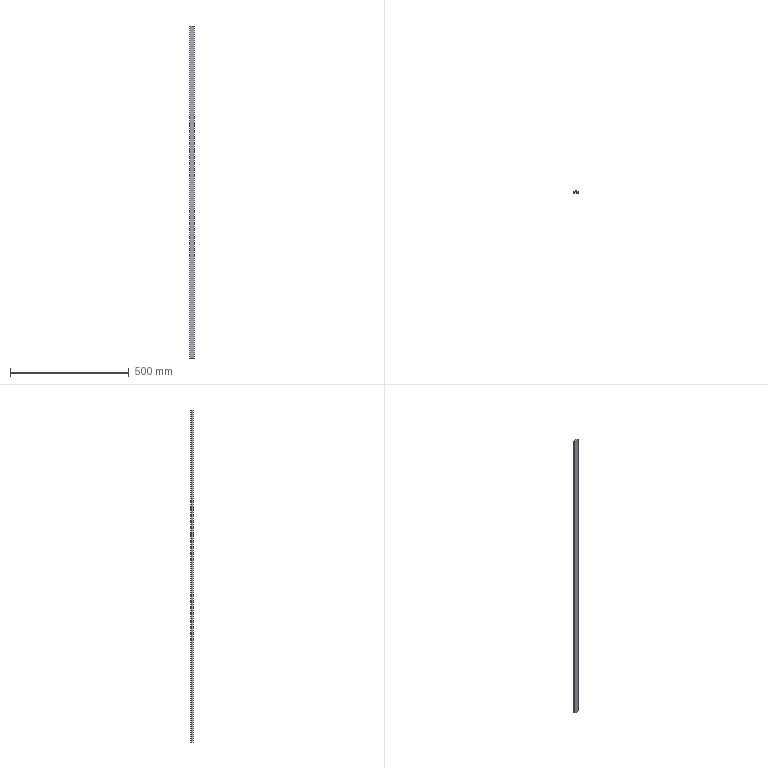Part | STEP file | GDT40-2000 | 1 solid | 10 faces | box 20 x 10 x 1400 mm | volume 237664 mm3 | plane 10
STEP:
#1=CARTESIAN_POINT('',(3.7,10.,400.));
#2=VERTEX_POINT('',#1);
#3=CARTESIAN_POINT('',(3.7,10.,-1000.));
#4=VERTEX_POINT('',#3);
#5=CARTESIAN_POINT('',(3.7,10.,1000.));
#6=DIRECTION('',(0.,0.,-1.));
#7=VECTOR('',#6,1000.);
#8=LINE('',#5,#7);
#9=EDGE_CURVE('',#2,#4,#8,.T.);
#10=ORIENTED_EDGE('',*,*,#9,.F.);
#11=CARTESIAN_POINT('',(3.7,7.6,400.));
#12=VERTEX_POINT('',#11);
#13=CARTESIAN_POINT('',(3.7,7.6,400.));
#14=DIRECTION('',(0.,1.,0.));
#15=VECTOR('',#14,1000.);
#16=LINE('',#13,#15);
#17=EDGE_CURVE('',#12,#2,#16,.T.);
#18=ORIENTED_EDGE('',*,*,#17,.F.);
#19=CARTESIAN_POINT('',(3.7,7.6,-1000.));
#20=VERTEX_POINT('',#19);
#21=CARTESIAN_POINT('',(3.7,7.6,1000.));
#22=DIRECTION('',(0.,0.,1.));
#23=VECTOR('',#22,1000.);
#24=LINE('',#21,#23);
#25=EDGE_CURVE('',#20,#12,#24,.T.);
#26=ORIENTED_EDGE('',*,*,#25,.F.);
#27=CARTESIAN_POINT('',(3.7,0.,-1000.));
#28=DIRECTION('',(0.,1.,0.));
#29=VECTOR('',#28,1000.);
#30=LINE('',#27,#29);
#31=EDGE_CURVE('',#20,#4,#30,.T.);
#32=ORIENTED_EDGE('',*,*,#31,.T.);
#33=EDGE_LOOP('',(#10,#18,#26,#32));
#34=FACE_OUTER_BOUND('',#33,.T.);
#35=CARTESIAN_POINT('',(3.7,7.6,1000.));
#36=DIRECTION('',(1.,0.,0.));
#37=DIRECTION('',(0.,0.,-1.));
#38=AXIS2_PLACEMENT_3D('',#35,#36,#37);
#39=PLANE('',#38);
#40=ADVANCED_FACE('',(#34),#39,.T.);
#41=CARTESIAN_POINT('',(-3.7,10.,400.));
#42=VERTEX_POINT('',#41);
#43=CARTESIAN_POINT('',(-3.7,10.,-1000.));
#44=VERTEX_POINT('',#43);
#45=CARTESIAN_POINT('',(-3.7,10.,1000.));
#46=DIRECTION('',(0.,0.,-1.));
#47=VECTOR('',#46,1000.);
#48=LINE('',#45,#47);
#49=EDGE_CURVE('',#42,#44,#48,.T.);
#50=ORIENTED_EDGE('',*,*,#49,.F.);
#51=CARTESIAN_POINT('',(3.7,10.,400.));
#52=DIRECTION('',(-1.,0.,0.));
#53=VECTOR('',#52,1000.);
#54=LINE('',#51,#53);
#55=EDGE_CURVE('',#2,#42,#54,.T.);
#56=ORIENTED_EDGE('',*,*,#55,.F.);
#57=ORIENTED_EDGE('',*,*,#9,.T.);
#58=CARTESIAN_POINT('',(0.,10.,-1000.));
#59=DIRECTION('',(-1.,0.,0.));
#60=VECTOR('',#59,1000.);
#61=LINE('',#58,#60);
#62=EDGE_CURVE('',#4,#44,#61,.T.);
#63=ORIENTED_EDGE('',*,*,#62,.T.);
#64=EDGE_LOOP('',(#50,#56,#57,#63));
#65=FACE_OUTER_BOUND('',#64,.T.);
#66=CARTESIAN_POINT('',(3.7,10.,1000.));
#67=DIRECTION('',(0.,1.,0.));
#68=DIRECTION('',(0.,0.,1.));
#69=AXIS2_PLACEMENT_3D('',#66,#67,#68);
#70=PLANE('',#69);
#71=ADVANCED_FACE('',(#65),#70,.T.);
#72=CARTESIAN_POINT('',(-3.7,7.6,400.));
#73=VERTEX_POINT('',#72);
#74=CARTESIAN_POINT('',(-3.7,7.6,-1000.));
#75=VERTEX_POINT('',#74);
#76=CARTESIAN_POINT('',(-3.7,7.6,1000.));
#77=DIRECTION('',(0.,0.,-1.));
#78=VECTOR('',#77,1000.);
#79=LINE('',#76,#78);
#80=EDGE_CURVE('',#73,#75,#79,.T.);
#81=ORIENTED_EDGE('',*,*,#80,.F.);
#82=CARTESIAN_POINT('',(-3.7,10.,400.));
#83=DIRECTION('',(0.,-1.,0.));
#84=VECTOR('',#83,1000.);
#85=LINE('',#82,#84);
#86=EDGE_CURVE('',#42,#73,#85,.T.);
#87=ORIENTED_EDGE('',*,*,#86,.F.);
#88=ORIENTED_EDGE('',*,*,#49,.T.);
#89=CARTESIAN_POINT('',(-3.7,0.,-1000.));
#90=DIRECTION('',(0.,-1.,0.));
#91=VECTOR('',#90,1000.);
#92=LINE('',#89,#91);
#93=EDGE_CURVE('',#44,#75,#92,.T.);
#94=ORIENTED_EDGE('',*,*,#93,.T.);
#95=EDGE_LOOP('',(#81,#87,#88,#94));
#96=FACE_OUTER_BOUND('',#95,.T.);
#97=CARTESIAN_POINT('',(-3.7,10.,1000.));
#98=DIRECTION('',(-1.,0.,0.));
#99=DIRECTION('',(0.,-1.,0.));
#100=AXIS2_PLACEMENT_3D('',#97,#98,#99);
#101=PLANE('',#100);
#102=ADVANCED_FACE('',(#96),#101,.T.);
#103=CARTESIAN_POINT('',(-10.,7.6,400.));
#104=VERTEX_POINT('',#103);
#105=CARTESIAN_POINT('',(-10.,7.6,-1000.));
#106=VERTEX_POINT('',#105);
#107=CARTESIAN_POINT('',(-10.,7.6,1000.));
#108=DIRECTION('',(0.,0.,-1.));
#109=VECTOR('',#108,1000.);
#110=LINE('',#107,#109);
#111=EDGE_CURVE('',#104,#106,#110,.T.);
#112=ORIENTED_EDGE('',*,*,#111,.F.);
#113=CARTESIAN_POINT('',(-3.7,7.6,400.));
#114=DIRECTION('',(-1.,0.,0.));
#115=VECTOR('',#114,1000.);
#116=LINE('',#113,#115);
#117=EDGE_CURVE('',#73,#104,#116,.T.);
#118=ORIENTED_EDGE('',*,*,#117,.F.);
#119=ORIENTED_EDGE('',*,*,#80,.T.);
#120=CARTESIAN_POINT('',(0.,7.6,-1000.));
#121=DIRECTION('',(-1.,0.,0.));
#122=VECTOR('',#121,1000.);
#123=LINE('',#120,#122);
#124=EDGE_CURVE('',#75,#106,#123,.T.);
#125=ORIENTED_EDGE('',*,*,#124,.T.);
#126=EDGE_LOOP('',(#112,#118,#119,#125));
#127=FACE_OUTER_BOUND('',#126,.T.);
#128=CARTESIAN_POINT('',(-3.7,7.6,1000.));
#129=DIRECTION('',(0.,1.,0.));
#130=DIRECTION('',(-1.,0.,0.));
#131=AXIS2_PLACEMENT_3D('',#128,#129,#130);
#132=PLANE('',#131);
#133=ADVANCED_FACE('',(#127),#132,.T.);
#134=ORIENTED_EDGE('',*,*,#25,.T.);
#135=CARTESIAN_POINT('',(10.,7.6,400.));
#136=VERTEX_POINT('',#135);
#137=CARTESIAN_POINT('',(10.,7.6,400.));
#138=DIRECTION('',(-1.,0.,0.));
#139=VECTOR('',#138,1000.);
#140=LINE('',#137,#139);
#141=EDGE_CURVE('',#136,#12,#140,.T.);
#142=ORIENTED_EDGE('',*,*,#141,.F.);
#143=CARTESIAN_POINT('',(10.,7.6,-1000.));
#144=VERTEX_POINT('',#143);
#145=CARTESIAN_POINT('',(10.,7.6,1000.));
#146=DIRECTION('',(0.,0.,1.));
#147=VECTOR('',#146,1000.);
#148=LINE('',#145,#147);
#149=EDGE_CURVE('',#144,#136,#148,.T.);
#150=ORIENTED_EDGE('',*,*,#149,.F.);
#151=CARTESIAN_POINT('',(0.,7.6,-1000.));
#152=DIRECTION('',(-1.,0.,0.));
#153=VECTOR('',#152,1000.);
#154=LINE('',#151,#153);
#155=EDGE_CURVE('',#144,#20,#154,.T.);
#156=ORIENTED_EDGE('',*,*,#155,.T.);
#157=EDGE_LOOP('',(#134,#142,#150,#156));
#158=FACE_OUTER_BOUND('',#157,.T.);
#159=CARTESIAN_POINT('',(10.,7.6,1000.));
#160=DIRECTION('',(0.,1.,0.));
#161=DIRECTION('',(-1.,0.,0.));
#162=AXIS2_PLACEMENT_3D('',#159,#160,#161);
#163=PLANE('',#162);
#164=ADVANCED_FACE('',(#158),#163,.T.);
#165=CARTESIAN_POINT('',(-10.,0.,400.));
#166=VERTEX_POINT('',#165);
#167=CARTESIAN_POINT('',(-10.,0.,-1000.));
#168=VERTEX_POINT('',#167);
#169=CARTESIAN_POINT('',(-10.,0.,1000.));
#170=DIRECTION('',(0.,0.,-1.));
#171=VECTOR('',#170,1000.);
#172=LINE('',#169,#171);
#173=EDGE_CURVE('',#166,#168,#172,.T.);
#174=ORIENTED_EDGE('',*,*,#173,.F.);
#175=CARTESIAN_POINT('',(-10.,7.6,400.));
#176=DIRECTION('',(0.,-1.,0.));
#177=VECTOR('',#176,1000.);
#178=LINE('',#175,#177);
#179=EDGE_CURVE('',#104,#166,#178,.T.);
#180=ORIENTED_EDGE('',*,*,#179,.F.);
#181=ORIENTED_EDGE('',*,*,#111,.T.);
#182=CARTESIAN_POINT('',(-10.,0.,-1000.));
#183=DIRECTION('',(0.,-1.,0.));
#184=VECTOR('',#183,1000.);
#185=LINE('',#182,#184);
#186=EDGE_CURVE('',#106,#168,#185,.T.);
#187=ORIENTED_EDGE('',*,*,#186,.T.);
#188=EDGE_LOOP('',(#174,#180,#181,#187));
#189=FACE_OUTER_BOUND('',#188,.T.);
#190=CARTESIAN_POINT('',(-10.,7.6,1000.));
#191=DIRECTION('',(-1.,0.,0.));
#192=DIRECTION('',(0.,0.,1.));
#193=AXIS2_PLACEMENT_3D('',#190,#191,#192);
#194=PLANE('',#193);
#195=ADVANCED_FACE('',(#189),#194,.T.);
#196=ORIENTED_EDGE('',*,*,#149,.T.);
#197=CARTESIAN_POINT('',(10.,0.,400.));
#198=VERTEX_POINT('',#197);
#199=CARTESIAN_POINT('',(10.,0.,400.));
#200=DIRECTION('',(0.,1.,0.));
#201=VECTOR('',#200,1000.);
#202=LINE('',#199,#201);
#203=EDGE_CURVE('',#198,#136,#202,.T.);
#204=ORIENTED_EDGE('',*,*,#203,.F.);
#205=CARTESIAN_POINT('',(10.,0.,-1000.));
#206=VERTEX_POINT('',#205);
#207=CARTESIAN_POINT('',(10.,0.,1000.));
#208=DIRECTION('',(0.,0.,1.));
#209=VECTOR('',#208,1000.);
#210=LINE('',#207,#209);
#211=EDGE_CURVE('',#206,#198,#210,.T.);
#212=ORIENTED_EDGE('',*,*,#211,.F.);
#213=CARTESIAN_POINT('',(10.,0.,-1000.));
#214=DIRECTION('',(0.,1.,0.));
#215=VECTOR('',#214,1000.);
#216=LINE('',#213,#215);
#217=EDGE_CURVE('',#206,#144,#216,.T.);
#218=ORIENTED_EDGE('',*,*,#217,.T.);
#219=EDGE_LOOP('',(#196,#204,#212,#218));
#220=FACE_OUTER_BOUND('',#219,.T.);
#221=CARTESIAN_POINT('',(10.,0.,1000.));
#222=DIRECTION('',(1.,0.,0.));
#223=DIRECTION('',(0.,0.,-1.));
#224=AXIS2_PLACEMENT_3D('',#221,#222,#223);
#225=PLANE('',#224);
#226=ADVANCED_FACE('',(#220),#225,.T.);
#227=ORIENTED_EDGE('',*,*,#211,.T.);
#228=CARTESIAN_POINT('',(-10.,0.,400.));
#229=DIRECTION('',(1.,0.,0.));
#230=VECTOR('',#229,1000.);
#231=LINE('',#228,#230);
#232=EDGE_CURVE('',#166,#198,#231,.T.);
#233=ORIENTED_EDGE('',*,*,#232,.F.);
#234=ORIENTED_EDGE('',*,*,#173,.T.);
#235=CARTESIAN_POINT('',(-10.,0.,-1000.));
#236=DIRECTION('',(1.,0.,0.));
#237=VECTOR('',#236,1000.);
#238=LINE('',#235,#237);
#239=EDGE_CURVE('',#168,#206,#238,.T.);
#240=ORIENTED_EDGE('',*,*,#239,.T.);
#241=EDGE_LOOP('',(#227,#233,#234,#240));
#242=FACE_OUTER_BOUND('',#241,.T.);
#243=CARTESIAN_POINT('',(-10.,0.,1000.));
#244=DIRECTION('',(0.,-1.,0.));
#245=DIRECTION('',(0.,0.,-1.));
#246=AXIS2_PLACEMENT_3D('',#243,#244,#245);
#247=PLANE('',#246);
#248=ADVANCED_FACE('',(#242),#247,.T.);
#249=ORIENTED_EDGE('',*,*,#186,.F.);
#250=ORIENTED_EDGE('',*,*,#124,.F.);
#251=ORIENTED_EDGE('',*,*,#93,.F.);
#252=ORIENTED_EDGE('',*,*,#62,.F.);
#253=ORIENTED_EDGE('',*,*,#31,.F.);
#254=ORIENTED_EDGE('',*,*,#155,.F.);
#255=ORIENTED_EDGE('',*,*,#217,.F.);
#256=ORIENTED_EDGE('',*,*,#239,.F.);
#257=EDGE_LOOP('',(#249,#250,#251,#252,#253,#254,#255,#256));
#258=FACE_OUTER_BOUND('',#257,.T.);
#259=CARTESIAN_POINT('',(0.,0.,-1000.));
#260=DIRECTION('',(0.,0.,1.));
#261=DIRECTION('',(1.,0.,0.));
#262=AXIS2_PLACEMENT_3D('',#259,#260,#261);
#263=PLANE('',#262);
#264=ADVANCED_FACE('',(#258),#263,.F.);
#265=ORIENTED_EDGE('',*,*,#17,.T.);
#266=ORIENTED_EDGE('',*,*,#55,.T.);
#267=ORIENTED_EDGE('',*,*,#86,.T.);
#268=ORIENTED_EDGE('',*,*,#117,.T.);
#269=ORIENTED_EDGE('',*,*,#179,.T.);
#270=ORIENTED_EDGE('',*,*,#232,.T.);
#271=ORIENTED_EDGE('',*,*,#203,.T.);
#272=ORIENTED_EDGE('',*,*,#141,.T.);
#273=EDGE_LOOP('',(#265,#266,#267,#268,#269,#270,#271,#272));
#274=FACE_OUTER_BOUND('',#273,.T.);
#275=CARTESIAN_POINT('',(0.,0.,400.));
#276=DIRECTION('',(0.,0.,1.));
#277=DIRECTION('',(1.,0.,0.));
#278=AXIS2_PLACEMENT_3D('',#275,#276,#277);
#279=PLANE('',#278);
#280=ADVANCED_FACE('',(#274),#279,.T.);
#281=CLOSED_SHELL('',(#40,#71,#102,#133,#164,#195,#226,#248,#264,#280));
#282=MANIFOLD_SOLID_BREP('',#281);
#283=CARTESIAN_POINT('',(0.,0.,0.));
#284=DIRECTION('',(0.,0.,1.));
#285=DIRECTION('',(1.,0.,0.));
#286=AXIS2_PLACEMENT_3D('',#283,#284,#285);
#287=(LENGTH_UNIT()NAMED_UNIT(*)SI_UNIT(.MILLI.,.METRE.));
#288=UNCERTAINTY_MEASURE_WITH_UNIT(LENGTH_MEASURE(0.00001),#287,'','');
#289=(NAMED_UNIT(*)PLANE_ANGLE_UNIT()SI_UNIT($,.RADIAN.));
#290=(NAMED_UNIT(*)SI_UNIT($,.STERADIAN.)SOLID_ANGLE_UNIT());
#291=(GEOMETRIC_REPRESENTATION_CONTEXT(3)GLOBAL_UNCERTAINTY_ASSIGNED_CONTEXT((#288))GLOBAL_UNIT_ASSIGNED_CONTEXT((#287,#289,#290))REPRESENTATION_CONTEXT('',''));
#292=ADVANCED_BREP_SHAPE_REPRESENTATION('',(#282,#286),#291);